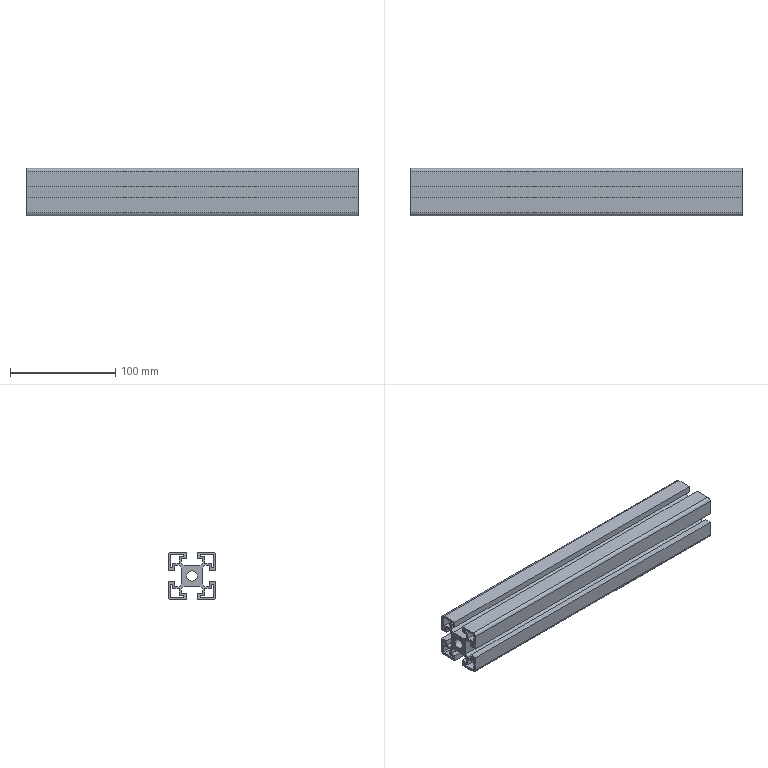Part | STEP file | 1_11 | 1 solid | 87 faces | box 315 x 45 x 45 mm | volume 257589 mm3 | plane 78 | cylinder 9 | commonest cylinder face diameters 2 x4 6 x4 10 x1